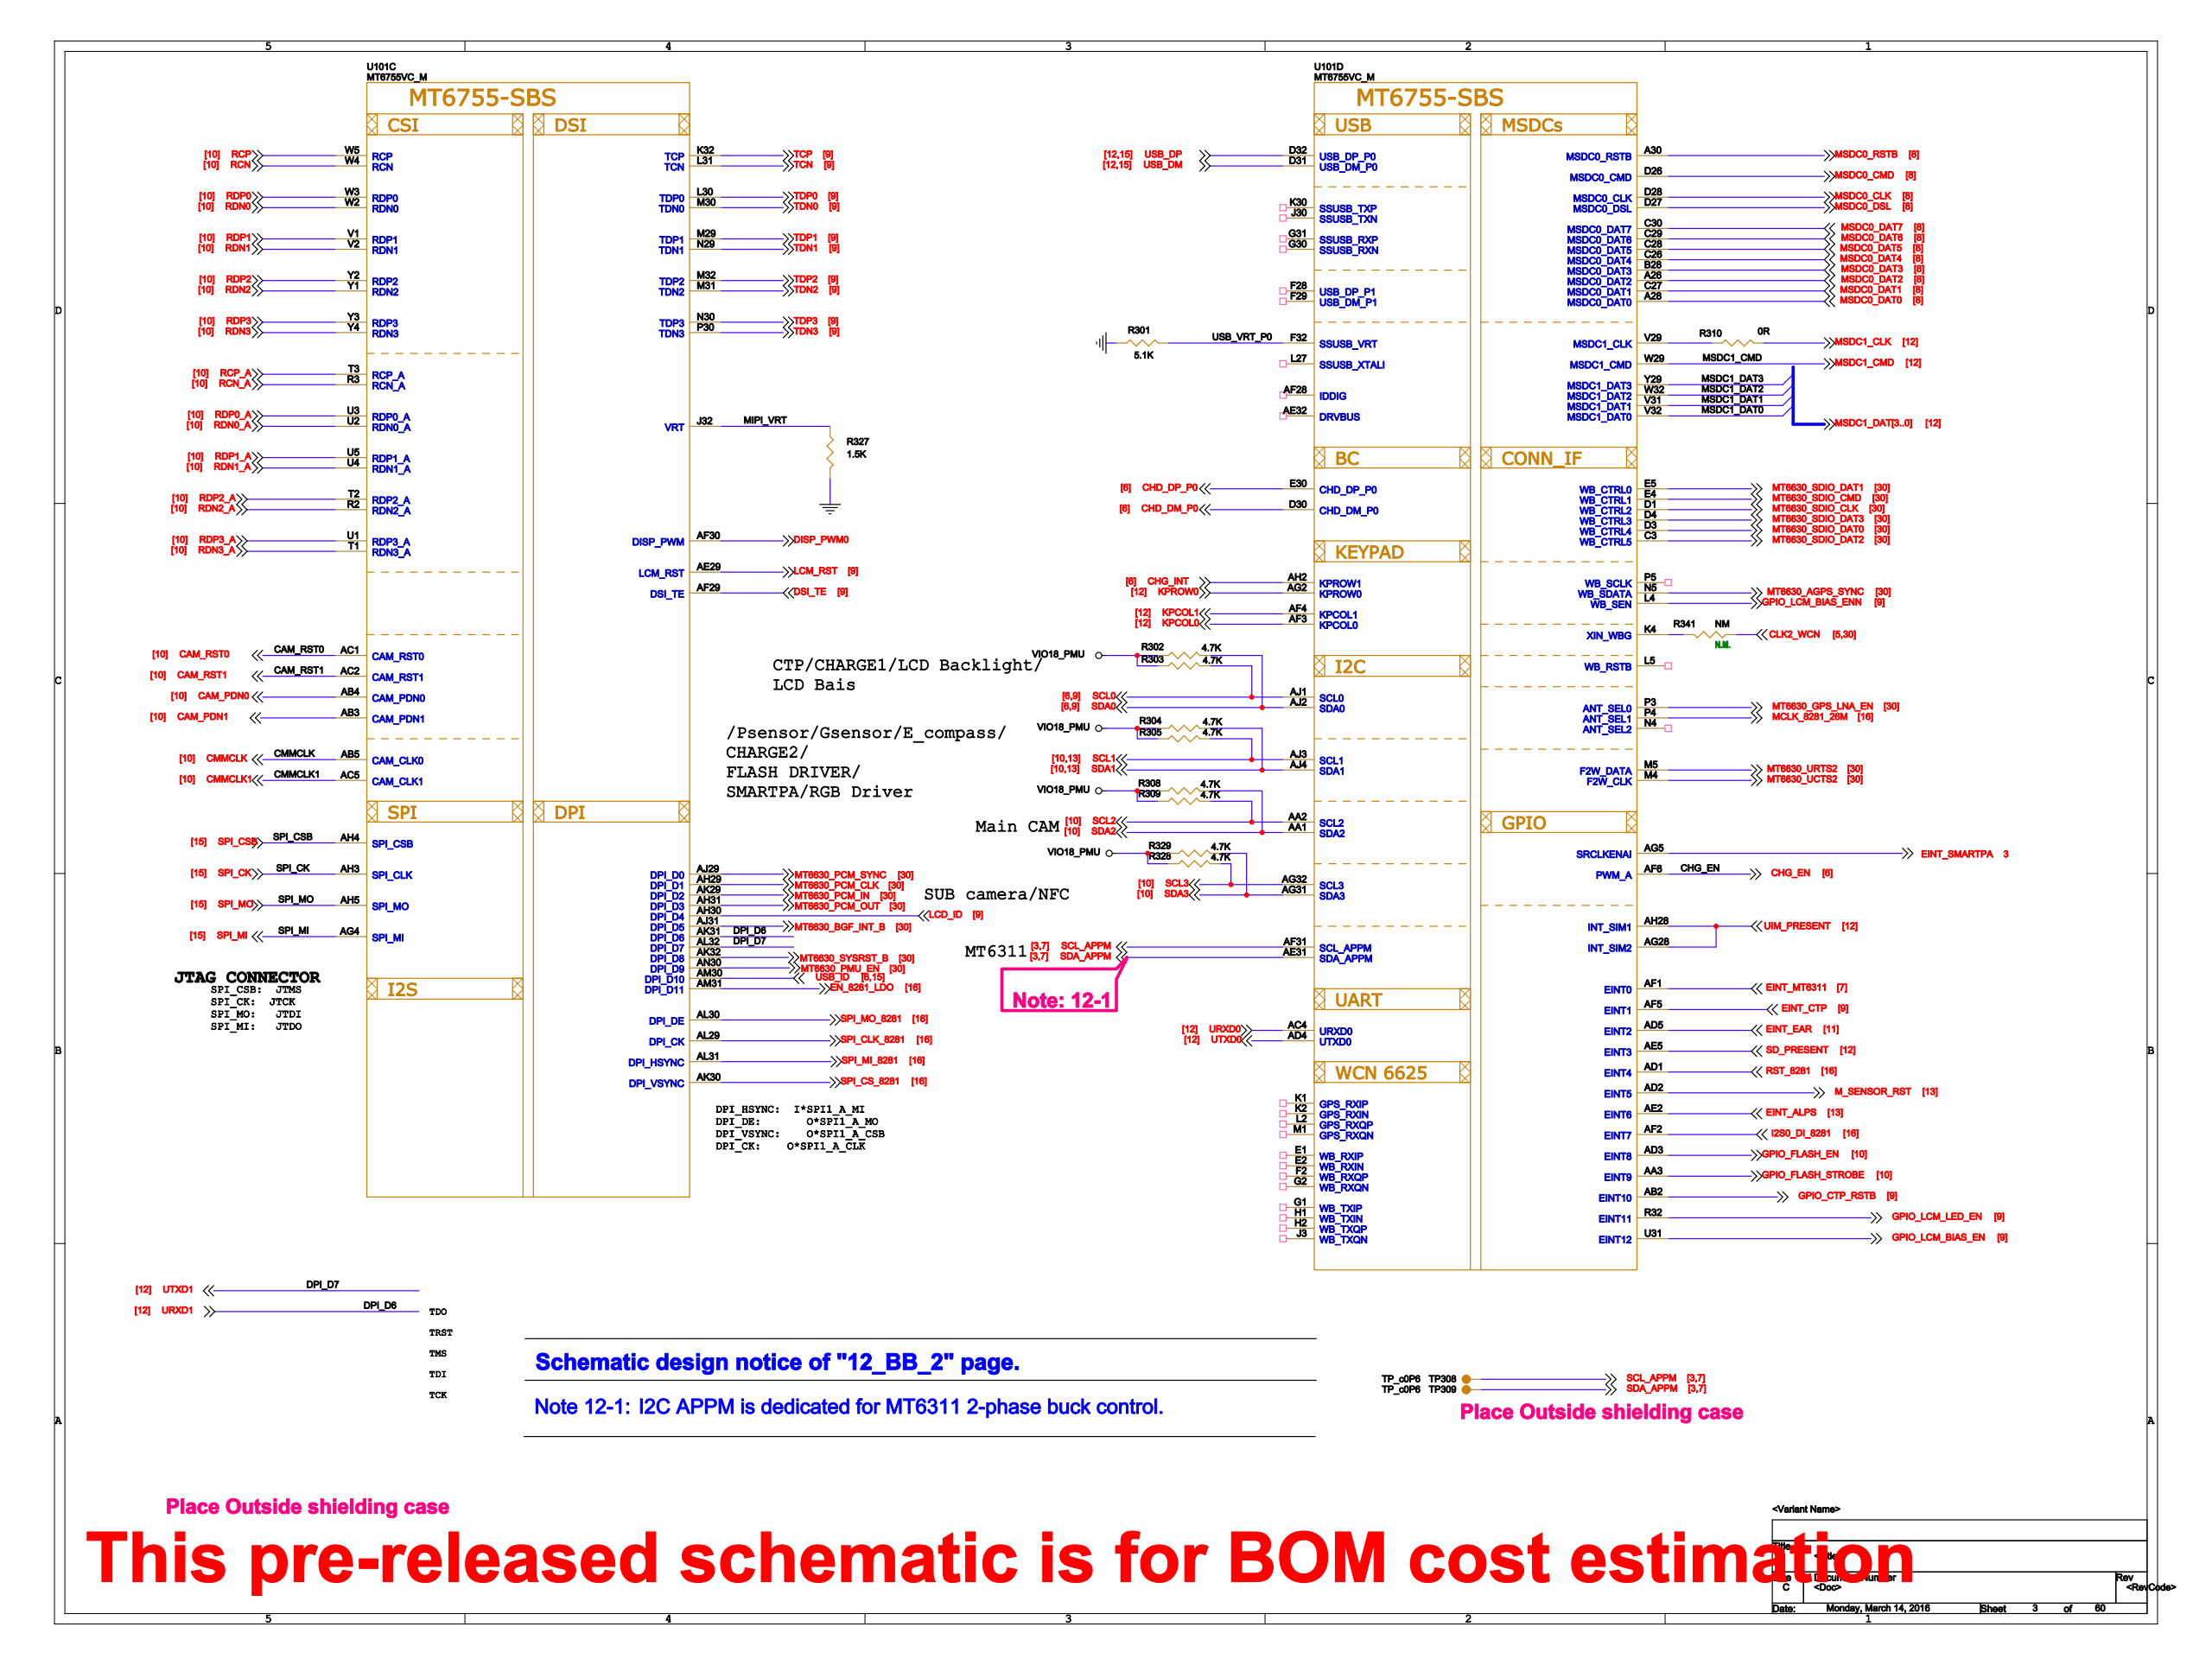Circuit board | Cadence Allegro | 1088 parts | 793 nets | one sheet of the schematic
Parts on this sheet (reference | value | footprint):
R301 | 5.1K | R0201
R302 | 4.7K | R0201
R303 | 4.7K | R0201
R304 | 4.7K | R0201
R305 | 4.7K | R0201
R308 | 4.7K | R0201
R309 | 4.7K | R0201
R310 | 0R | R0201
R327 | 1.5K | R0201
R328 | 4.7K | R0201
R329 | 4.7K | R0201
R341
TP308 | TP_c0P6 | TP_C0P6
TP309 | TP_c0P6 | TP_C0P6
U101 | MT6755VC_M | MT6755
Nets of these parts (net: part-pin ...):
GND: R301-2 R327-2
EINT_ALPS: U101-AE2
SCL1: R305-2 U101-AJ3
SDA1: R304-2 U101-AJ4
MT6630_GPS_LNA_EN: U101-P3
CMMCLK: U101-AB5
CMMCLK1: U101-AC5
CAM_PDN0: U101-AB4
CAM_PDN1: U101-AB3
CAM_RST0: U101-AC1
CAM_RST1: U101-AC2
DISP_PWM0: U101-AF30
SPI_CLK_8281: U101-AL29
MT6630_PCM_SYNC: U101-AJ29
MT6630_PCM_CLK: U101-AH29
USB_ID: U101-AM30
EN_8281_LDO: U101-AM31
MT6630_PCM_IN: U101-AK29
MT6630_PCM_OUT: U101-AH31
LCD_ID: U101-AH30
MT6630_BGF_INT_B: U101-AJ31
URXD1: U101-AK31
UTXD1: U101-AL32
MT6630_SYSRST_B: U101-AK32
MT6630_PMU_EN: U101-AN30
SPI_MO_8281: U101-AL30
SPI_MI_8281: U101-AL31
SPI_CS_8281: U101-AK30
DSI_TE: U101-AF29
LCM_RST: U101-AE29
RCN: U101-W4
RCN_A: U101-R3
RCP: U101-W5
RCP_A: U101-T3
RDN0: U101-W2
RDN0_A: U101-U2
RDN1: U101-V2
RDN1_A: U101-U4
RDN2: U101-Y1
RDN2_A: U101-R2
RDN3: U101-Y4
RDN3_A: U101-T1
RDP0: U101-W3
RDP0_A: U101-U3
RDP1: U101-V1
RDP1_A: U101-U5
RDP2: U101-Y2
RDP2_A: U101-T2
RDP3: U101-Y3
RDP3_A: U101-U1
SPI_CK: U101-AH3
SPI_CSB: U101-AH4
SPI_MI: U101-AG4
SPI_MO: U101-AH5
TCN: U101-L31
TCP: U101-K32
TDN0: U101-M30
TDN1: U101-N29
TDN2: U101-M31
TDN3: U101-P30
TDP0: U101-L30
TDP1: U101-M29
TDP2: U101-M32
TDP3: U101-N30
MIPI_VRT: R327-1 U101-J32
MCLK_8281_26M: U101-P4
CHD_DM_P0: U101-D30
CHD_DP_P0: U101-E30
EINT_MT6311: U101-AF1
EINT_CTP: U101-AF5
GPIO_CTP_RSTB: U101-AB2
GPIO_LCM_LED_EN: U101-R32
GPIO_LCM_BIAS_EN: U101-U31
EINT_EAR: U101-AD5
SD_PRESENT: U101-AE5
RST_8281: U101-AD1
M_SENSOR_RST: U101-AD2
I2S0_DI_8281: U101-AF2
GPIO_FLASH_EN: U101-AD3
GPIO_FLASH_STROBE: U101-AA3
MT6630_UCTS2: U101-M4
MT6630_URTS2: U101-M5
UIM_PRESENT: U101-AG28 U101-AH28
KPCOL0: U101-AF3
KPCOL1: U101-AF4
KPROW0: U101-AG2
CHG_INT: U101-AH2
MSDC0_CLK: U101-D28
MSDC0_CMD: U101-D26
MSDC0_DAT0: U101-A28
MSDC0_DAT1: U101-C27
MSDC0_DAT2: U101-A26
MSDC0_DAT3: U101-B28
MSDC0_DAT4: U101-C26
MSDC0_DAT5: U101-C28
MSDC0_DAT6: U101-C29
MSDC0_DAT7: U101-C30
MSDC0_DSL: U101-D27
MSDC0_RSTB: U101-A30
N35043493: R310-1 U101-V29
MSDC1_CMD: U101-W29
MSDC1_DAT0: U101-V32
MSDC1_DAT1: U101-V31
MSDC1_DAT2: U101-W32
MSDC1_DAT3: U101-Y29
CHG_EN: U101-AF6
SCL0: R303-2 U101-AJ1
SCL2: R309-2 U101-AA2
SCL3: R328-2 U101-AG32
SCL_APPM: TP308-1 U101-AF31
SDA0: R302-2 U101-AJ2
SDA2: R308-2 U101-AA1
SDA3: R329-2 U101-AG31
SDA_APPM: TP309-1 U101-AE31
EINT_SMARTPA: U101-AG5
USB_VRT_P0: R301-1 U101-F32
URXD0: U101-AC4
USB_DM: U101-D31
USB_DP: U101-D32
UTXD0: U101-AD4
MT6630_SDIO_DAT1: U101-E5
MT6630_SDIO_CMD: U101-E4
MT6630_SDIO_CLK: U101-D1
MT6630_SDIO_DAT3: U101-D4
MT6630_SDIO_DAT0: U101-D3
MT6630_SDIO_DAT2: U101-C3
MT6630_AGPS_SYNC: U101-N5
GPIO_LCM_BIAS_ENN: U101-L4
N33778155: R341-2 U101-K4
VIO18_PMU: R302-1 R303-1 R304-1 R305-1 R308-1 R309-1 R328-1 R329-1
MSDC1_CLK: R310-2
CLK2_WCN: R341-1